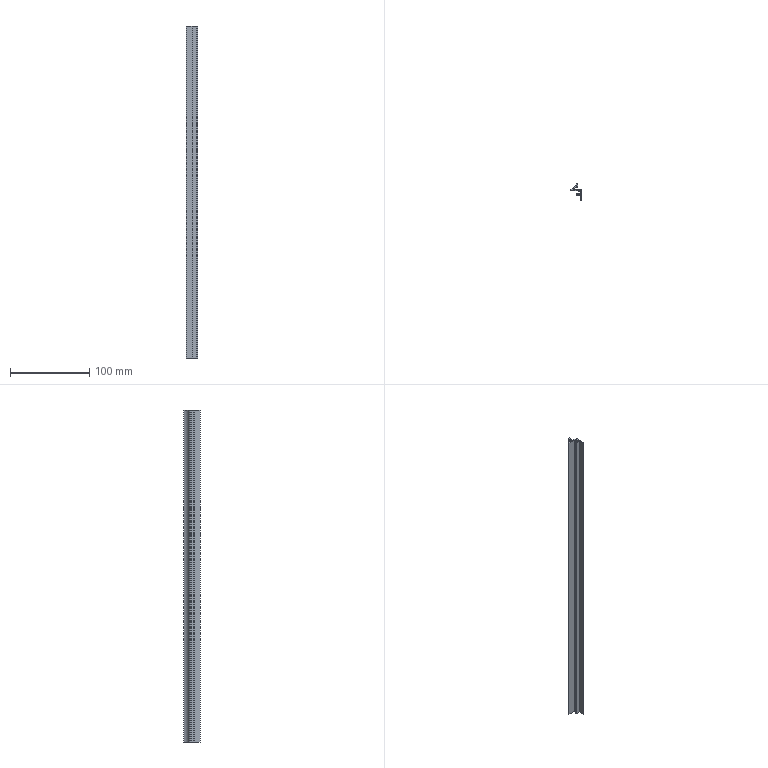Part | SolidWorks | features BaseBody 1, ICE 1, MoveFace 1 | 1 solid | 27 faces | box 14 x 20.3 x 420 mm | volume 21385 mm3 | plane 20 | cylinder 7 | commonest cylinder face diameters 0.387 x2 0.8 x2 0.4 x1 20 x1 22 x1
STEP:
#1=CARTESIAN_POINT('',(-5.304,-0.625,200.));
#2=VERTEX_POINT('',#1);
#3=CARTESIAN_POINT('',(-5.449,-0.8125,200.));
#4=VERTEX_POINT('',#3);
#5=CARTESIAN_POINT('',(-5.255,-0.8125,200.));
#6=DIRECTION('',(0.,0.,1.));
#7=DIRECTION('',(-1.,0.,0.));
#8=AXIS2_PLACEMENT_3D('',#5,#6,#7);
#9=CIRCLE('',#8,0.1937);
#10=EDGE_CURVE('',#2,#4,#9,.T.);
#11=ORIENTED_EDGE('',*,*,#10,.T.);
#12=CARTESIAN_POINT('',(-5.449,-0.8125,-220.));
#13=VERTEX_POINT('',#12);
#14=CARTESIAN_POINT('',(-5.449,-0.8125,230.));
#15=DIRECTION('',(0.,0.,-1.));
#16=VECTOR('',#15,1000.);
#17=LINE('',#14,#16);
#18=EDGE_CURVE('',#4,#13,#17,.T.);
#19=ORIENTED_EDGE('',*,*,#18,.T.);
#20=CARTESIAN_POINT('',(-5.304,-0.625,-220.));
#21=VERTEX_POINT('',#20);
#22=CARTESIAN_POINT('',(-5.255,-0.8125,-220.));
#23=DIRECTION('',(0.,0.,-1.));
#24=DIRECTION('',(1.,0.,0.));
#25=AXIS2_PLACEMENT_3D('',#22,#23,#24);
#26=CIRCLE('',#25,0.1937);
#27=EDGE_CURVE('',#13,#21,#26,.T.);
#28=ORIENTED_EDGE('',*,*,#27,.T.);
#29=CARTESIAN_POINT('',(-5.304,-0.625,230.));
#30=DIRECTION('',(0.,0.,-1.));
#31=VECTOR('',#30,1000.);
#32=LINE('',#29,#31);
#33=EDGE_CURVE('',#2,#21,#32,.T.);
#34=ORIENTED_EDGE('',*,*,#33,.F.);
#35=EDGE_LOOP('',(#11,#19,#28,#34));
#36=FACE_OUTER_BOUND('',#35,.T.);
#37=CARTESIAN_POINT('',(-5.255,-0.8125,230.));
#38=DIRECTION('',(0.,0.,-1.));
#39=DIRECTION('',(-1.,0.,0.));
#40=AXIS2_PLACEMENT_3D('',#37,#38,#39);
#41=CYLINDRICAL_SURFACE('',#40,0.1937);
#42=ADVANCED_FACE('',(#36),#41,.F.);
#43=CARTESIAN_POINT('',(5.,-1.,-220.));
#44=VERTEX_POINT('',#43);
#45=CARTESIAN_POINT('',(5.,-14.3,-220.));
#46=VERTEX_POINT('',#45);
#47=CARTESIAN_POINT('',(5.,29.623,-220.));
#48=DIRECTION('',(0.,-1.,0.));
#49=VECTOR('',#48,1000.);
#50=LINE('',#47,#49);
#51=EDGE_CURVE('',#44,#46,#50,.T.);
#52=ORIENTED_EDGE('',*,*,#51,.F.);
#53=CARTESIAN_POINT('',(5.,-1.,200.));
#54=VERTEX_POINT('',#53);
#55=CARTESIAN_POINT('',(5.,-1.,230.));
#56=DIRECTION('',(0.,0.,-1.));
#57=VECTOR('',#56,1000.);
#58=LINE('',#55,#57);
#59=EDGE_CURVE('',#54,#44,#58,.T.);
#60=ORIENTED_EDGE('',*,*,#59,.F.);
#61=CARTESIAN_POINT('',(5.,-14.3,200.));
#62=VERTEX_POINT('',#61);
#63=CARTESIAN_POINT('',(5.,-14.3,200.));
#64=DIRECTION('',(0.,1.,0.));
#65=VECTOR('',#64,1000.);
#66=LINE('',#63,#65);
#67=EDGE_CURVE('',#62,#54,#66,.T.);
#68=ORIENTED_EDGE('',*,*,#67,.F.);
#69=CARTESIAN_POINT('',(5.,-14.3,230.));
#70=DIRECTION('',(0.,0.,1.));
#71=VECTOR('',#70,1000.);
#72=LINE('',#69,#71);
#73=EDGE_CURVE('',#46,#62,#72,.T.);
#74=ORIENTED_EDGE('',*,*,#73,.F.);
#75=EDGE_LOOP('',(#52,#60,#68,#74));
#76=FACE_OUTER_BOUND('',#75,.T.);
#77=CARTESIAN_POINT('',(5.,-14.3,230.));
#78=DIRECTION('',(-1.,0.,0.));
#79=DIRECTION('',(0.,0.,1.));
#80=AXIS2_PLACEMENT_3D('',#77,#78,#79);
#81=PLANE('',#80);
#82=ADVANCED_FACE('',(#76),#81,.F.);
#83=CARTESIAN_POINT('',(-9.,-2.,-220.));
#84=VERTEX_POINT('',#83);
#85=CARTESIAN_POINT('',(-9.,-2.,200.));
#86=VERTEX_POINT('',#85);
#87=CARTESIAN_POINT('',(-9.,-2.,230.));
#88=DIRECTION('',(0.,0.,1.));
#89=VECTOR('',#88,1000.);
#90=LINE('',#87,#89);
#91=EDGE_CURVE('',#84,#86,#90,.T.);
#92=ORIENTED_EDGE('',*,*,#91,.F.);
#93=CARTESIAN_POINT('',(0.9,-2.,-220.));
#94=VERTEX_POINT('',#93);
#95=CARTESIAN_POINT('',(5.,-2.,-220.));
#96=DIRECTION('',(-1.,0.,0.));
#97=VECTOR('',#96,1000.);
#98=LINE('',#95,#97);
#99=EDGE_CURVE('',#94,#84,#98,.T.);
#100=ORIENTED_EDGE('',*,*,#99,.F.);
#101=CARTESIAN_POINT('',(0.9,-2.,200.));
#102=VERTEX_POINT('',#101);
#103=CARTESIAN_POINT('',(0.9,-2.,230.));
#104=DIRECTION('',(0.,0.,-1.));
#105=VECTOR('',#104,1000.);
#106=LINE('',#103,#105);
#107=EDGE_CURVE('',#102,#94,#106,.T.);
#108=ORIENTED_EDGE('',*,*,#107,.F.);
#109=CARTESIAN_POINT('',(5.,-2.,200.));
#110=DIRECTION('',(1.,0.,0.));
#111=VECTOR('',#110,1000.);
#112=LINE('',#109,#111);
#113=EDGE_CURVE('',#86,#102,#112,.T.);
#114=ORIENTED_EDGE('',*,*,#113,.F.);
#115=EDGE_LOOP('',(#92,#100,#108,#114));
#116=FACE_OUTER_BOUND('',#115,.T.);
#117=CARTESIAN_POINT('',(-9.,-2.,230.));
#118=DIRECTION('',(0.,1.,0.));
#119=DIRECTION('',(0.,0.,1.));
#120=AXIS2_PLACEMENT_3D('',#117,#118,#119);
#121=PLANE('',#120);
#122=ADVANCED_FACE('',(#116),#121,.F.);
#123=CARTESIAN_POINT('',(4.,-6.,200.));
#124=VERTEX_POINT('',#123);
#125=CARTESIAN_POINT('',(4.,-3.,200.));
#126=VERTEX_POINT('',#125);
#127=CARTESIAN_POINT('',(4.,29.623,200.));
#128=DIRECTION('',(0.,1.,0.));
#129=VECTOR('',#128,1000.);
#130=LINE('',#127,#129);
#131=EDGE_CURVE('',#124,#126,#130,.T.);
#132=ORIENTED_EDGE('',*,*,#131,.F.);
#133=CARTESIAN_POINT('',(1.,-6.,200.));
#134=VERTEX_POINT('',#133);
#135=CARTESIAN_POINT('',(5.,-6.,200.));
#136=DIRECTION('',(1.,0.,0.));
#137=VECTOR('',#136,1000.);
#138=LINE('',#135,#137);
#139=EDGE_CURVE('',#134,#124,#138,.T.);
#140=ORIENTED_EDGE('',*,*,#139,.F.);
#141=CARTESIAN_POINT('',(1.,-6.7,200.));
#142=VERTEX_POINT('',#141);
#143=CARTESIAN_POINT('',(1.,-6.,200.));
#144=DIRECTION('',(0.,-1.,0.));
#145=VECTOR('',#144,1000.);
#146=LINE('',#143,#145);
#147=EDGE_CURVE('',#134,#142,#146,.T.);
#148=ORIENTED_EDGE('',*,*,#147,.T.);
#149=CARTESIAN_POINT('',(-1.7,-6.7,200.));
#150=VERTEX_POINT('',#149);
#151=CARTESIAN_POINT('',(5.,-6.7,200.));
#152=DIRECTION('',(1.,0.,0.));
#153=VECTOR('',#152,1000.);
#154=LINE('',#151,#153);
#155=EDGE_CURVE('',#150,#142,#154,.T.);
#156=ORIENTED_EDGE('',*,*,#155,.F.);
#157=CARTESIAN_POINT('',(-1.7,-7.7,200.));
#158=VERTEX_POINT('',#157);
#159=CARTESIAN_POINT('',(-1.7,-6.7,200.));
#160=DIRECTION('',(0.,-1.,0.));
#161=VECTOR('',#160,1000.);
#162=LINE('',#159,#161);
#163=EDGE_CURVE('',#150,#158,#162,.T.);
#164=ORIENTED_EDGE('',*,*,#163,.T.);
#165=CARTESIAN_POINT('',(4.,-7.7,200.));
#166=VERTEX_POINT('',#165);
#167=CARTESIAN_POINT('',(5.,-7.7,200.));
#168=DIRECTION('',(-1.,0.,0.));
#169=VECTOR('',#168,1000.);
#170=LINE('',#167,#169);
#171=EDGE_CURVE('',#166,#158,#170,.T.);
#172=ORIENTED_EDGE('',*,*,#171,.F.);
#173=CARTESIAN_POINT('',(4.,-14.3,200.));
#174=VERTEX_POINT('',#173);
#175=CARTESIAN_POINT('',(4.,29.623,200.));
#176=DIRECTION('',(0.,1.,0.));
#177=VECTOR('',#176,1000.);
#178=LINE('',#175,#177);
#179=EDGE_CURVE('',#174,#166,#178,.T.);
#180=ORIENTED_EDGE('',*,*,#179,.F.);
#181=CARTESIAN_POINT('',(5.,-14.3,200.));
#182=DIRECTION('',(-1.,0.,0.));
#183=VECTOR('',#182,1000.);
#184=LINE('',#181,#183);
#185=EDGE_CURVE('',#62,#174,#184,.T.);
#186=ORIENTED_EDGE('',*,*,#185,.F.);
#187=ORIENTED_EDGE('',*,*,#67,.T.);
#188=CARTESIAN_POINT('',(-5.207,-1.,200.));
#189=VERTEX_POINT('',#188);
#190=CARTESIAN_POINT('',(5.,-1.,200.));
#191=DIRECTION('',(1.,0.,0.));
#192=VECTOR('',#191,1000.);
#193=LINE('',#190,#192);
#194=EDGE_CURVE('',#189,#54,#193,.T.);
#195=ORIENTED_EDGE('',*,*,#194,.F.);
#196=CARTESIAN_POINT('',(-5.255,-0.8125,200.));
#197=DIRECTION('',(0.,0.,1.));
#198=DIRECTION('',(-1.,0.,0.));
#199=AXIS2_PLACEMENT_3D('',#196,#197,#198);
#200=CIRCLE('',#199,0.1937);
#201=EDGE_CURVE('',#4,#189,#200,.T.);
#202=ORIENTED_EDGE('',*,*,#201,.F.);
#203=ORIENTED_EDGE('',*,*,#10,.F.);
#204=CARTESIAN_POINT('',(-1.368,3.063,200.));
#205=VERTEX_POINT('',#204);
#206=CARTESIAN_POINT('',(-10.628,9.,200.));
#207=DIRECTION('',(0.,0.,1.));
#208=DIRECTION('',(-1.,0.,0.));
#209=AXIS2_PLACEMENT_3D('',#206,#207,#208);
#210=CIRCLE('',#209,11.);
#211=EDGE_CURVE('',#2,#205,#210,.T.);
#212=ORIENTED_EDGE('',*,*,#211,.T.);
#213=CARTESIAN_POINT('',(-1.,2.955,200.));
#214=VERTEX_POINT('',#213);
#215=CARTESIAN_POINT('',(-1.2,2.955,200.));
#216=DIRECTION('',(0.,0.,1.));
#217=DIRECTION('',(-1.,0.,0.));
#218=AXIS2_PLACEMENT_3D('',#215,#216,#217);
#219=CIRCLE('',#218,0.2);
#220=EDGE_CURVE('',#214,#205,#219,.T.);
#221=ORIENTED_EDGE('',*,*,#220,.F.);
#222=CARTESIAN_POINT('',(-1.,1.5,200.));
#223=VERTEX_POINT('',#222);
#224=CARTESIAN_POINT('',(-1.,2.955,200.));
#225=DIRECTION('',(0.,1.,0.));
#226=VECTOR('',#225,1000.);
#227=LINE('',#224,#226);
#228=EDGE_CURVE('',#223,#214,#227,.T.);
#229=ORIENTED_EDGE('',*,*,#228,.F.);
#230=CARTESIAN_POINT('',(0.,1.5,200.));
#231=VERTEX_POINT('',#230);
#232=CARTESIAN_POINT('',(-1.,1.5,200.));
#233=DIRECTION('',(-1.,0.,0.));
#234=VECTOR('',#233,1000.);
#235=LINE('',#232,#234);
#236=EDGE_CURVE('',#231,#223,#235,.T.);
#237=ORIENTED_EDGE('',*,*,#236,.F.);
#238=CARTESIAN_POINT('',(0.,6.,200.));
#239=VERTEX_POINT('',#238);
#240=CARTESIAN_POINT('',(0.,1.5,200.));
#241=DIRECTION('',(0.,-1.,0.));
#242=VECTOR('',#241,1000.);
#243=LINE('',#240,#242);
#244=EDGE_CURVE('',#239,#231,#243,.T.);
#245=ORIENTED_EDGE('',*,*,#244,.F.);
#246=CARTESIAN_POINT('',(-0.8,6.,200.));
#247=VERTEX_POINT('',#246);
#248=CARTESIAN_POINT('',(0.,6.,200.));
#249=DIRECTION('',(1.,0.,0.));
#250=VECTOR('',#249,1000.);
#251=LINE('',#248,#250);
#252=EDGE_CURVE('',#247,#239,#251,.T.);
#253=ORIENTED_EDGE('',*,*,#252,.F.);
#254=CARTESIAN_POINT('',(-1.178,5.731,200.));
#255=VERTEX_POINT('',#254);
#256=CARTESIAN_POINT('',(-0.8,5.6,200.));
#257=DIRECTION('',(0.,0.,1.));
#258=DIRECTION('',(-1.,0.,0.));
#259=AXIS2_PLACEMENT_3D('',#256,#257,#258);
#260=CIRCLE('',#259,0.4);
#261=EDGE_CURVE('',#247,#255,#260,.T.);
#262=ORIENTED_EDGE('',*,*,#261,.T.);
#263=CARTESIAN_POINT('',(-8.678,-0.8077,200.));
#264=VERTEX_POINT('',#263);
#265=CARTESIAN_POINT('',(-10.628,9.,200.));
#266=DIRECTION('',(0.,0.,1.));
#267=DIRECTION('',(-1.,0.,0.));
#268=AXIS2_PLACEMENT_3D('',#265,#266,#267);
#269=CIRCLE('',#268,10.);
#270=EDGE_CURVE('',#264,#255,#269,.T.);
#271=ORIENTED_EDGE('',*,*,#270,.F.);
#272=CARTESIAN_POINT('',(-9.,-1.2,200.));
#273=VERTEX_POINT('',#272);
#274=CARTESIAN_POINT('',(-8.6,-1.2,200.));
#275=DIRECTION('',(0.,0.,1.));
#276=DIRECTION('',(-1.,0.,0.));
#277=AXIS2_PLACEMENT_3D('',#274,#275,#276);
#278=CIRCLE('',#277,0.4);
#279=EDGE_CURVE('',#264,#273,#278,.T.);
#280=ORIENTED_EDGE('',*,*,#279,.T.);
#281=CARTESIAN_POINT('',(-9.,8.,200.));
#282=DIRECTION('',(0.,-1.,0.));
#283=VECTOR('',#282,1000.);
#284=LINE('',#281,#283);
#285=EDGE_CURVE('',#273,#86,#284,.T.);
#286=ORIENTED_EDGE('',*,*,#285,.T.);
#287=ORIENTED_EDGE('',*,*,#113,.T.);
#288=CARTESIAN_POINT('',(0.9,-3.,200.));
#289=VERTEX_POINT('',#288);
#290=CARTESIAN_POINT('',(0.9,29.623,200.));
#291=DIRECTION('',(0.,1.,0.));
#292=VECTOR('',#291,1000.);
#293=LINE('',#290,#292);
#294=EDGE_CURVE('',#289,#102,#293,.T.);
#295=ORIENTED_EDGE('',*,*,#294,.F.);
#296=CARTESIAN_POINT('',(5.,-3.,200.));
#297=DIRECTION('',(-1.,0.,0.));
#298=VECTOR('',#297,1000.);
#299=LINE('',#296,#298);
#300=EDGE_CURVE('',#126,#289,#299,.T.);
#301=ORIENTED_EDGE('',*,*,#300,.F.);
#302=EDGE_LOOP('',(#132,#140,#148,#156,#164,#172,#180,#186,#187,#195,#202,#203,#212,#221,#229,#237,#245,#253,#262,#271,#280,#286,#287,#295,#301));
#303=FACE_OUTER_BOUND('',#302,.T.);
#304=CARTESIAN_POINT('',(5.,29.623,200.));
#305=DIRECTION('',(0.,0.,-1.));
#306=DIRECTION('',(-1.,0.,0.));
#307=AXIS2_PLACEMENT_3D('',#304,#305,#306);
#308=PLANE('',#307);
#309=ADVANCED_FACE('',(#303),#308,.F.);
#310=ORIENTED_EDGE('',*,*,#185,.T.);
#311=CARTESIAN_POINT('',(4.,-14.3,-220.));
#312=VERTEX_POINT('',#311);
#313=CARTESIAN_POINT('',(4.,-14.3,230.));
#314=DIRECTION('',(0.,0.,1.));
#315=VECTOR('',#314,1000.);
#316=LINE('',#313,#315);
#317=EDGE_CURVE('',#312,#174,#316,.T.);
#318=ORIENTED_EDGE('',*,*,#317,.F.);
#319=CARTESIAN_POINT('',(5.,-14.3,-220.));
#320=DIRECTION('',(-1.,0.,0.));
#321=VECTOR('',#320,1000.);
#322=LINE('',#319,#321);
#323=EDGE_CURVE('',#46,#312,#322,.T.);
#324=ORIENTED_EDGE('',*,*,#323,.F.);
#325=ORIENTED_EDGE('',*,*,#73,.T.);
#326=EDGE_LOOP('',(#310,#318,#324,#325));
#327=FACE_OUTER_BOUND('',#326,.T.);
#328=CARTESIAN_POINT('',(4.,-14.3,230.));
#329=DIRECTION('',(0.,1.,0.));
#330=DIRECTION('',(0.,0.,1.));
#331=AXIS2_PLACEMENT_3D('',#328,#329,#330);
#332=PLANE('',#331);
#333=ADVANCED_FACE('',(#327),#332,.F.);
#334=ORIENTED_EDGE('',*,*,#51,.T.);
#335=ORIENTED_EDGE('',*,*,#323,.T.);
#336=CARTESIAN_POINT('',(4.,-7.7,-220.));
#337=VERTEX_POINT('',#336);
#338=CARTESIAN_POINT('',(4.,-7.7,-220.));
#339=DIRECTION('',(0.,-1.,0.));
#340=VECTOR('',#339,1000.);
#341=LINE('',#338,#340);
#342=EDGE_CURVE('',#337,#312,#341,.T.);
#343=ORIENTED_EDGE('',*,*,#342,.F.);
#344=CARTESIAN_POINT('',(-1.7,-7.7,-220.));
#345=VERTEX_POINT('',#344);
#346=CARTESIAN_POINT('',(-1.7,-7.7,-220.));
#347=DIRECTION('',(1.,0.,0.));
#348=VECTOR('',#347,1000.);
#349=LINE('',#346,#348);
#350=EDGE_CURVE('',#345,#337,#349,.T.);
#351=ORIENTED_EDGE('',*,*,#350,.F.);
#352=CARTESIAN_POINT('',(-1.7,-6.7,-220.));
#353=VERTEX_POINT('',#352);
#354=CARTESIAN_POINT('',(-1.7,29.623,-220.));
#355=DIRECTION('',(0.,1.,0.));
#356=VECTOR('',#355,1000.);
#357=LINE('',#354,#356);
#358=EDGE_CURVE('',#345,#353,#357,.T.);
#359=ORIENTED_EDGE('',*,*,#358,.T.);
#360=CARTESIAN_POINT('',(1.,-6.7,-220.));
#361=VERTEX_POINT('',#360);
#362=CARTESIAN_POINT('',(1.,-6.7,-220.));
#363=DIRECTION('',(-1.,0.,0.));
#364=VECTOR('',#363,1000.);
#365=LINE('',#362,#364);
#366=EDGE_CURVE('',#361,#353,#365,.T.);
#367=ORIENTED_EDGE('',*,*,#366,.F.);
#368=CARTESIAN_POINT('',(1.,-6.,-220.));
#369=VERTEX_POINT('',#368);
#370=CARTESIAN_POINT('',(1.,29.623,-220.));
#371=DIRECTION('',(0.,1.,0.));
#372=VECTOR('',#371,1000.);
#373=LINE('',#370,#372);
#374=EDGE_CURVE('',#361,#369,#373,.T.);
#375=ORIENTED_EDGE('',*,*,#374,.T.);
#376=CARTESIAN_POINT('',(4.,-6.,-220.));
#377=VERTEX_POINT('',#376);
#378=CARTESIAN_POINT('',(4.,-6.,-220.));
#379=DIRECTION('',(-1.,0.,0.));
#380=VECTOR('',#379,1000.);
#381=LINE('',#378,#380);
#382=EDGE_CURVE('',#377,#369,#381,.T.);
#383=ORIENTED_EDGE('',*,*,#382,.F.);
#384=CARTESIAN_POINT('',(4.,-3.,-220.));
#385=VERTEX_POINT('',#384);
#386=CARTESIAN_POINT('',(4.,-3.,-220.));
#387=DIRECTION('',(0.,-1.,0.));
#388=VECTOR('',#387,1000.);
#389=LINE('',#386,#388);
#390=EDGE_CURVE('',#385,#377,#389,.T.);
#391=ORIENTED_EDGE('',*,*,#390,.F.);
#392=CARTESIAN_POINT('',(0.9,-3.,-220.));
#393=VERTEX_POINT('',#392);
#394=CARTESIAN_POINT('',(0.9,-3.,-220.));
#395=DIRECTION('',(1.,0.,0.));
#396=VECTOR('',#395,1000.);
#397=LINE('',#394,#396);
#398=EDGE_CURVE('',#393,#385,#397,.T.);
#399=ORIENTED_EDGE('',*,*,#398,.F.);
#400=CARTESIAN_POINT('',(0.9,-2.,-220.));
#401=DIRECTION('',(0.,-1.,0.));
#402=VECTOR('',#401,1000.);
#403=LINE('',#400,#402);
#404=EDGE_CURVE('',#94,#393,#403,.T.);
#405=ORIENTED_EDGE('',*,*,#404,.F.);
#406=ORIENTED_EDGE('',*,*,#99,.T.);
#407=CARTESIAN_POINT('',(-9.,-1.2,-220.));
#408=VERTEX_POINT('',#407);
#409=CARTESIAN_POINT('',(-9.,-1.2,-220.));
#410=DIRECTION('',(0.,-1.,0.));
#411=VECTOR('',#410,1000.);
#412=LINE('',#409,#411);
#413=EDGE_CURVE('',#408,#84,#412,.T.);
#414=ORIENTED_EDGE('',*,*,#413,.F.);
#415=CARTESIAN_POINT('',(-8.678,-0.8077,-220.));
#416=VERTEX_POINT('',#415);
#417=CARTESIAN_POINT('',(-8.6,-1.2,-220.));
#418=DIRECTION('',(0.,0.,-1.));
#419=DIRECTION('',(1.,0.,0.));
#420=AXIS2_PLACEMENT_3D('',#417,#418,#419);
#421=CIRCLE('',#420,0.4);
#422=EDGE_CURVE('',#408,#416,#421,.T.);
#423=ORIENTED_EDGE('',*,*,#422,.T.);
#424=CARTESIAN_POINT('',(-1.178,5.731,-220.));
#425=VERTEX_POINT('',#424);
#426=CARTESIAN_POINT('',(-10.628,9.,-220.));
#427=DIRECTION('',(0.,0.,-1.));
#428=DIRECTION('',(1.,0.,0.));
#429=AXIS2_PLACEMENT_3D('',#426,#427,#428);
#430=CIRCLE('',#429,10.);
#431=EDGE_CURVE('',#425,#416,#430,.T.);
#432=ORIENTED_EDGE('',*,*,#431,.F.);
#433=CARTESIAN_POINT('',(-0.8,6.,-220.));
#434=VERTEX_POINT('',#433);
#435=CARTESIAN_POINT('',(-0.8,5.6,-220.));
#436=DIRECTION('',(0.,0.,-1.));
#437=DIRECTION('',(1.,0.,0.));
#438=AXIS2_PLACEMENT_3D('',#435,#436,#437);
#439=CIRCLE('',#438,0.4);
#440=EDGE_CURVE('',#425,#434,#439,.T.);
#441=ORIENTED_EDGE('',*,*,#440,.T.);
#442=CARTESIAN_POINT('',(0.,6.,-220.));
#443=VERTEX_POINT('',#442);
#444=CARTESIAN_POINT('',(0.,6.,-220.));
#445=DIRECTION('',(-1.,0.,0.));
#446=VECTOR('',#445,1000.);
#447=LINE('',#444,#446);
#448=EDGE_CURVE('',#443,#434,#447,.T.);
#449=ORIENTED_EDGE('',*,*,#448,.F.);
#450=CARTESIAN_POINT('',(0.,1.5,-220.));
#451=VERTEX_POINT('',#450);
#452=CARTESIAN_POINT('',(0.,1.5,-220.));
#453=DIRECTION('',(0.,1.,0.));
#454=VECTOR('',#453,1000.);
#455=LINE('',#452,#454);
#456=EDGE_CURVE('',#451,#443,#455,.T.);
#457=ORIENTED_EDGE('',*,*,#456,.F.);
#458=CARTESIAN_POINT('',(-1.,1.5,-220.));
#459=VERTEX_POINT('',#458);
#460=CARTESIAN_POINT('',(-1.,1.5,-220.));
#461=DIRECTION('',(1.,0.,0.));
#462=VECTOR('',#461,1000.);
#463=LINE('',#460,#462);
#464=EDGE_CURVE('',#459,#451,#463,.T.);
#465=ORIENTED_EDGE('',*,*,#464,.F.);
#466=CARTESIAN_POINT('',(-1.,2.955,-220.));
#467=VERTEX_POINT('',#466);
#468=CARTESIAN_POINT('',(-1.,2.955,-220.));
#469=DIRECTION('',(0.,-1.,0.));
#470=VECTOR('',#469,1000.);
#471=LINE('',#468,#470);
#472=EDGE_CURVE('',#467,#459,#471,.T.);
#473=ORIENTED_EDGE('',*,*,#472,.F.);
#474=CARTESIAN_POINT('',(-1.368,3.063,-220.));
#475=VERTEX_POINT('',#474);
#476=CARTESIAN_POINT('',(-1.2,2.955,-220.));
#477=DIRECTION('',(0.,0.,-1.));
#478=DIRECTION('',(1.,0.,0.));
#479=AXIS2_PLACEMENT_3D('',#476,#477,#478);
#480=CIRCLE('',#479,0.2);
#481=EDGE_CURVE('',#475,#467,#480,.T.);
#482=ORIENTED_EDGE('',*,*,#481,.F.);
#483=CARTESIAN_POINT('',(-10.628,9.,-220.));
#484=DIRECTION('',(0.,0.,-1.));
#485=DIRECTION('',(1.,0.,0.));
#486=AXIS2_PLACEMENT_3D('',#483,#484,#485);
#487=CIRCLE('',#486,11.);
#488=EDGE_CURVE('',#475,#21,#487,.T.);
#489=ORIENTED_EDGE('',*,*,#488,.T.);
#490=ORIENTED_EDGE('',*,*,#27,.F.);
#491=CARTESIAN_POINT('',(-5.207,-1.,-220.));
#492=VERTEX_POINT('',#491);
#493=CARTESIAN_POINT('',(-5.255,-0.8125,-220.));
#494=DIRECTION('',(0.,0.,-1.));
#495=DIRECTION('',(1.,0.,0.));
#496=AXIS2_PLACEMENT_3D('',#493,#494,#495);
#497=CIRCLE('',#496,0.1937);
#498=EDGE_CURVE('',#492,#13,#497,.T.);
#499=ORIENTED_EDGE('',*,*,#498,.F.);
#500=CARTESIAN_POINT('',(5.,-1.,-220.));
#501=DIRECTION('',(-1.,0.,0.));
#502=VECTOR('',#501,1000.);
#503=LINE('',#500,#502);
#504=EDGE_CURVE('',#44,#492,#503,.T.);
#505=ORIENTED_EDGE('',*,*,#504,.F.);
#506=EDGE_LOOP('',(#334,#335,#343,#351,#359,#367,#375,#383,#391,#399,#405,#406,#414,#423,#432,#441,#449,#457,#465,#473,#482,#489,#490,#499,#505));
#507=FACE_OUTER_BOUND('',#506,.T.);
#508=CARTESIAN_POINT('',(5.,29.623,-220.));
#509=DIRECTION('',(0.,0.,1.));
#510=DIRECTION('',(1.,0.,0.));
#511=AXIS2_PLACEMENT_3D('',#508,#509,#510);
#512=PLANE('',#511);
#513=ADVANCED_FACE('',(#507),#512,.F.);
#514=ORIENTED_EDGE('',*,*,#59,.T.);
#515=ORIENTED_EDGE('',*,*,#504,.T.);
#516=CARTESIAN_POINT('',(-5.207,-1.,230.));
#517=DIRECTION('',(0.,0.,-1.));
#518=VECTOR('',#517,1000.);
#519=LINE('',#516,#518);
#520=EDGE_CURVE('',#189,#492,#519,.T.);
#521=ORIENTED_EDGE('',*,*,#520,.F.);
#522=ORIENTED_EDGE('',*,*,#194,.T.);
#523=EDGE_LOOP('',(#514,#515,#521,#522));
#524=FACE_OUTER_BOUND('',#523,.T.);
#525=CARTESIAN_POINT('',(5.,-1.,230.));
#526=DIRECTION('',(0.,-1.,0.));
#527=DIRECTION('',(0.,0.,-1.));
#528=AXIS2_PLACEMENT_3D('',#525,#526,#527);
#529=PLANE('',#528);
#530=ADVANCED_FACE('',(#524),#529,.F.);
#531=CARTESIAN_POINT('',(-9.,-1.2,230.));
#532=DIRECTION('',(0.,0.,1.));
#533=VECTOR('',#532,1000.);
#534=LINE('',#531,#533);
#535=EDGE_CURVE('',#408,#273,#534,.T.);
#536=ORIENTED_EDGE('',*,*,#535,.F.);
#537=ORIENTED_EDGE('',*,*,#413,.T.);
#538=ORIENTED_EDGE('',*,*,#91,.T.);
#539=ORIENTED_EDGE('',*,*,#285,.F.);
#540=EDGE_LOOP('',(#536,#537,#538,#539));
#541=FACE_OUTER_BOUND('',#540,.T.);
#542=CARTESIAN_POINT('',(-9.,-1.2,230.));
#543=DIRECTION('',(1.,0.,0.));
#544=DIRECTION('',(0.,0.,-1.));
#545=AXIS2_PLACEMENT_3D('',#542,#543,#544);
#546=PLANE('',#545);
#547=ADVANCED_FACE('',(#541),#546,.F.);
#548=ORIENTED_EDGE('',*,*,#294,.T.);
#549=ORIENTED_EDGE('',*,*,#107,.T.);
#550=ORIENTED_EDGE('',*,*,#404,.T.);
#551=CARTESIAN_POINT('',(0.9,-3.,230.));
#552=DIRECTION('',(0.,0.,-1.));
#553=VECTOR('',#552,1000.);
#554=LINE('',#551,#553);
#555=EDGE_CURVE('',#289,#393,#554,.T.);
#556=ORIENTED_EDGE('',*,*,#555,.F.);
#557=EDGE_LOOP('',(#548,#549,#550,#556));
#558=FACE_OUTER_BOUND('',#557,.T.);
#559=CARTESIAN_POINT('',(0.9,-2.,230.));
#560=DIRECTION('',(1.,0.,0.));
#561=DIRECTION('',(0.,0.,-1.));
#562=AXIS2_PLACEMENT_3D('',#559,#560,#561);
#563=PLANE('',#562);
#564=ADVANCED_FACE('',(#558),#563,.F.);
#565=ORIENTED_EDGE('',*,*,#300,.T.);
#566=ORIENTED_EDGE('',*,*,#555,.T.);
#567=ORIENTED_EDGE('',*,*,#398,.T.);
#568=CARTESIAN_POINT('',(4.,-3.,230.));
#569=DIRECTION('',(0.,0.,-1.));
#570=VECTOR('',#569,1000.);
#571=LINE('',#568,#570);
#572=EDGE_CURVE('',#126,#385,#571,.T.);
#573=ORIENTED_EDGE('',*,*,#572,.F.);
#574=EDGE_LOOP('',(#565,#566,#567,#573));
#575=FACE_OUTER_BOUND('',#574,.T.);
#576=CARTESIAN_POINT('',(0.9,-3.,230.));
#577=DIRECTION('',(0.,1.,0.));
#578=DIRECTION('',(0.,0.,1.));
#579=AXIS2_PLACEMENT_3D('',#576,#577,#578);
#580=PLANE('',#579);
#581=ADVANCED_FACE('',(#575),#580,.F.);
#582=ORIENTED_EDGE('',*,*,#131,.T.);
#583=ORIENTED_EDGE('',*,*,#572,.T.);
#584=ORIENTED_EDGE('',*,*,#390,.T.);
#585=CARTESIAN_POINT('',(4.,-6.,230.));
#586=DIRECTION('',(0.,0.,-1.));
#587=VECTOR('',#586,1000.);
#588=LINE('',#585,#587);
#589=EDGE_CURVE('',#124,#377,#588,.T.);
#590=ORIENTED_EDGE('',*,*,#589,.F.);
#591=EDGE_LOOP('',(#582,#583,#584,#590));
#592=FACE_OUTER_BOUND('',#591,.T.);
#593=CARTESIAN_POINT('',(4.,-3.,230.));
#594=DIRECTION('',(1.,0.,0.));
#595=DIRECTION('',(0.,0.,-1.));
#596=AXIS2_PLACEMENT_3D('',#593,#594,#595);
#597=PLANE('',#596);
#598=ADVANCED_FACE('',(#592),#597,.F.);
#599=ORIENTED_EDGE('',*,*,#139,.T.);
#600=ORIENTED_EDGE('',*,*,#589,.T.);
#601=ORIENTED_EDGE('',*,*,#382,.T.);
#602=CARTESIAN_POINT('',(1.,-6.,230.));
#603=DIRECTION('',(0.,0.,-1.));
#604=VECTOR('',#603,1000.);
#605=LINE('',#602,#604);
#606=EDGE_CURVE('',#134,#369,#605,.T.);
#607=ORIENTED_EDGE('',*,*,#606,.F.);
#608=EDGE_LOOP('',(#599,#600,#601,#607));
#609=FACE_OUTER_BOUND('',#608,.T.);
#610=CARTESIAN_POINT('',(4.,-6.,230.));
#611=DIRECTION('',(0.,-1.,0.));
#612=DIRECTION('',(0.,0.,-1.));
#613=AXIS2_PLACEMENT_3D('',#610,#611,#612);
#614=PLANE('',#613);
#615=ADVANCED_FACE('',(#609),#614,.F.);
#616=ORIENTED_EDGE('',*,*,#155,.T.);
#617=CARTESIAN_POINT('',(1.,-6.7,230.));
#618=DIRECTION('',(0.,0.,1.));
#619=VECTOR('',#618,1000.);
#620=LINE('',#617,#619);
#621=EDGE_CURVE('',#361,#142,#620,.T.);
#622=ORIENTED_EDGE('',*,*,#621,.F.);
#623=ORIENTED_EDGE('',*,*,#366,.T.);
#624=CARTESIAN_POINT('',(-1.7,-6.7,230.));
#625=DIRECTION('',(0.,0.,-1.));
#626=VECTOR('',#625,1000.);
#627=LINE('',#624,#626);
#628=EDGE_CURVE('',#150,#353,#627,.T.);
#629=ORIENTED_EDGE('',*,*,#628,.F.);
#630=EDGE_LOOP('',(#616,#622,#623,#629));
#631=FACE_OUTER_BOUND('',#630,.T.);
#632=CARTESIAN_POINT('',(1.,-6.7,230.));
#633=DIRECTION('',(0.,-1.,0.));
#634=DIRECTION('',(0.,0.,-1.));
#635=AXIS2_PLACEMENT_3D('',#632,#633,#634);
#636=PLANE('',#635);
#637=ADVANCED_FACE('',(#631),#636,.F.);
#638=ORIENTED_EDGE('',*,*,#171,.T.);
#639=CARTESIAN_POINT('',(-1.7,-7.7,230.));
#640=DIRECTION('',(0.,0.,1.));
#641=VECTOR('',#640,1000.);
#642=LINE('',#639,#641);
#643=EDGE_CURVE('',#345,#158,#642,.T.);
#644=ORIENTED_EDGE('',*,*,#643,.F.);
#645=ORIENTED_EDGE('',*,*,#350,.T.);
#646=CARTESIAN_POINT('',(4.,-7.7,230.));
#647=DIRECTION('',(0.,0.,-1.));
#648=VECTOR('',#647,1000.);
#649=LINE('',#646,#648);
#650=EDGE_CURVE('',#166,#337,#649,.T.);
#651=ORIENTED_EDGE('',*,*,#650,.F.);
#652=EDGE_LOOP('',(#638,#644,#645,#651));
#653=FACE_OUTER_BOUND('',#652,.T.);
#654=CARTESIAN_POINT('',(-1.7,-7.7,230.));
#655=DIRECTION('',(0.,1.,0.));
#656=DIRECTION('',(0.,0.,1.));
#657=AXIS2_PLACEMENT_3D('',#654,#655,#656);
#658=PLANE('',#657);
#659=ADVANCED_FACE('',(#653),#658,.F.);
#660=ORIENTED_EDGE('',*,*,#179,.T.);
#661=ORIENTED_EDGE('',*,*,#650,.T.);
#662=ORIENTED_EDGE('',*,*,#342,.T.);
#663=ORIENTED_EDGE('',*,*,#317,.T.);
#664=EDGE_LOOP('',(#660,#661,#662,#663));
#665=FACE_OUTER_BOUND('',#664,.T.);
#666=CARTESIAN_POINT('',(4.,-7.7,230.));
#667=DIRECTION('',(1.,0.,0.));
#668=DIRECTION('',(0.,0.,-1.));
#669=AXIS2_PLACEMENT_3D('',#666,#667,#668);
#670=PLANE('',#669);
#671=ADVANCED_FACE('',(#665),#670,.F.);
#672=ORIENTED_EDGE('',*,*,#18,.F.);
#673=ORIENTED_EDGE('',*,*,#201,.T.);
#674=ORIENTED_EDGE('',*,*,#520,.T.);
#675=ORIENTED_EDGE('',*,*,#498,.T.);
#676=EDGE_LOOP('',(#672,#673,#674,#675));
#677=FACE_OUTER_BOUND('',#676,.T.);
#678=CARTESIAN_POINT('',(-5.255,-0.8125,230.));
#679=DIRECTION('',(0.,0.,-1.));
#680=DIRECTION('',(-1.,0.,0.));
#681=AXIS2_PLACEMENT_3D('',#678,#679,#680);
#682=CYLINDRICAL_SURFACE('',#681,0.1937);
#683=ADVANCED_FACE('',(#677),#682,.F.);
#684=CARTESIAN_POINT('',(-1.,2.955,230.));
#685=DIRECTION('',(0.,0.,1.));
#686=VECTOR('',#685,1000.);
#687=LINE('',#684,#686);
#688=EDGE_CURVE('',#467,#214,#687,.T.);
#689=ORIENTED_EDGE('',*,*,#688,.F.);
#690=ORIENTED_EDGE('',*,*,#472,.T.);
#691=CARTESIAN_POINT('',(-1.,1.5,230.));
#692=DIRECTION('',(0.,0.,-1.));
#693=VECTOR('',#692,1000.);
#694=LINE('',#691,#693);
#695=EDGE_CURVE('',#223,#459,#694,.T.);
#696=ORIENTED_EDGE('',*,*,#695,.F.);
#697=ORIENTED_EDGE('',*,*,#228,.T.);
#698=EDGE_LOOP('',(#689,#690,#696,#697));
#699=FACE_OUTER_BOUND('',#698,.T.);
#700=CARTESIAN_POINT('',(-1.,2.955,230.));
#701=DIRECTION('',(1.,0.,0.));
#702=DIRECTION('',(0.,0.,-1.));
#703=AXIS2_PLACEMENT_3D('',#700,#701,#702);
#704=PLANE('',#703);
#705=ADVANCED_FACE('',(#699),#704,.F.);
#706=ORIENTED_EDGE('',*,*,#488,.F.);
#707=CARTESIAN_POINT('',(-1.368,3.063,230.));
#708=DIRECTION('',(0.,0.,1.));
#709=VECTOR('',#708,1000.);
#710=LINE('',#707,#709);
#711=EDGE_CURVE('',#475,#205,#710,.T.);
#712=ORIENTED_EDGE('',*,*,#711,.T.);
#713=ORIENTED_EDGE('',*,*,#211,.F.);
#714=ORIENTED_EDGE('',*,*,#33,.T.);
#715=EDGE_LOOP('',(#706,#712,#713,#714));
#716=FACE_OUTER_BOUND('',#715,.T.);
#717=CARTESIAN_POINT('',(-10.628,9.,230.));
#718=DIRECTION('',(0.,0.,-1.));
#719=DIRECTION('',(-1.,0.,0.));
#720=AXIS2_PLACEMENT_3D('',#717,#718,#719);
#721=CYLINDRICAL_SURFACE('',#720,11.);
#722=ADVANCED_FACE('',(#716),#721,.T.);
#723=CARTESIAN_POINT('',(-1.178,5.731,230.));
#724=DIRECTION('',(0.,0.,1.));
#725=VECTOR('',#724,1000.);
#726=LINE('',#723,#725);
#727=EDGE_CURVE('',#425,#255,#726,.T.);
#728=ORIENTED_EDGE('',*,*,#727,.F.);
#729=ORIENTED_EDGE('',*,*,#431,.T.);
#730=CARTESIAN_POINT('',(-8.678,-0.8077,230.));
#731=DIRECTION('',(0.,0.,-1.));
#732=VECTOR('',#731,1000.);
#733=LINE('',#730,#732);
#734=EDGE_CURVE('',#264,#416,#733,.T.);
#735=ORIENTED_EDGE('',*,*,#734,.F.);
#736=ORIENTED_EDGE('',*,*,#270,.T.);
#737=EDGE_LOOP('',(#728,#729,#735,#736));
#738=FACE_OUTER_BOUND('',#737,.T.);
#739=CARTESIAN_POINT('',(-10.628,9.,230.));
#740=DIRECTION('',(0.,0.,-1.));
#741=DIRECTION('',(-1.,0.,0.));
#742=AXIS2_PLACEMENT_3D('',#739,#740,#741);
#743=CYLINDRICAL_SURFACE('',#742,10.);
#744=ADVANCED_FACE('',(#738),#743,.F.);
#745=CARTESIAN_POINT('',(0.,1.5,230.));
#746=DIRECTION('',(0.,0.,1.));
#747=VECTOR('',#746,1000.);
#748=LINE('',#745,#747);
#749=EDGE_CURVE('',#451,#231,#748,.T.);
#750=ORIENTED_EDGE('',*,*,#749,.F.);
#751=ORIENTED_EDGE('',*,*,#456,.T.);
#752=CARTESIAN_POINT('',(0.,6.,230.));
#753=DIRECTION('',(0.,0.,-1.));
#754=VECTOR('',#753,1000.);
#755=LINE('',#752,#754);
#756=EDGE_CURVE('',#239,#443,#755,.T.);
#757=ORIENTED_EDGE('',*,*,#756,.F.);
#758=ORIENTED_EDGE('',*,*,#244,.T.);
#759=EDGE_LOOP('',(#750,#751,#757,#758));
#760=FACE_OUTER_BOUND('',#759,.T.);
#761=CARTESIAN_POINT('',(0.,1.5,230.));
#762=DIRECTION('',(-1.,0.,0.));
#763=DIRECTION('',(0.,0.,1.));
#764=AXIS2_PLACEMENT_3D('',#761,#762,#763);
#765=PLANE('',#764);
#766=ADVANCED_FACE('',(#760),#765,.F.);
#767=ORIENTED_EDGE('',*,*,#422,.F.);
#768=ORIENTED_EDGE('',*,*,#535,.T.);
#769=ORIENTED_EDGE('',*,*,#279,.F.);
#770=ORIENTED_EDGE('',*,*,#734,.T.);
#771=EDGE_LOOP('',(#767,#768,#769,#770));
#772=FACE_OUTER_BOUND('',#771,.T.);
#773=CARTESIAN_POINT('',(-8.6,-1.2,230.));
#774=DIRECTION('',(0.,0.,-1.));
#775=DIRECTION('',(-1.,0.,0.));
#776=AXIS2_PLACEMENT_3D('',#773,#774,#775);
#777=CYLINDRICAL_SURFACE('',#776,0.4);
#778=ADVANCED_FACE('',(#772),#777,.T.);
#779=ORIENTED_EDGE('',*,*,#147,.F.);
#780=ORIENTED_EDGE('',*,*,#606,.T.);
#781=ORIENTED_EDGE('',*,*,#374,.F.);
#782=ORIENTED_EDGE('',*,*,#621,.T.);
#783=EDGE_LOOP('',(#779,#780,#781,#782));
#784=FACE_OUTER_BOUND('',#783,.T.);
#785=CARTESIAN_POINT('',(1.,-6.,230.));
#786=DIRECTION('',(1.,0.,0.));
#787=DIRECTION('',(0.,0.,-1.));
#788=AXIS2_PLACEMENT_3D('',#785,#786,#787);
#789=PLANE('',#788);
#790=ADVANCED_FACE('',(#784),#789,.F.);
#791=ORIENTED_EDGE('',*,*,#163,.F.);
#792=ORIENTED_EDGE('',*,*,#628,.T.);
#793=ORIENTED_EDGE('',*,*,#358,.F.);
#794=ORIENTED_EDGE('',*,*,#643,.T.);
#795=EDGE_LOOP('',(#791,#792,#793,#794));
#796=FACE_OUTER_BOUND('',#795,.T.);
#797=CARTESIAN_POINT('',(-1.7,-6.7,230.));
#798=DIRECTION('',(1.,0.,0.));
#799=DIRECTION('',(0.,0.,-1.));
#800=AXIS2_PLACEMENT_3D('',#797,#798,#799);
#801=PLANE('',#800);
#802=ADVANCED_FACE('',(#796),#801,.F.);
#803=ORIENTED_EDGE('',*,*,#711,.F.);
#804=ORIENTED_EDGE('',*,*,#481,.T.);
#805=ORIENTED_EDGE('',*,*,#688,.T.);
#806=ORIENTED_EDGE('',*,*,#220,.T.);
#807=EDGE_LOOP('',(#803,#804,#805,#806));
#808=FACE_OUTER_BOUND('',#807,.T.);
#809=CARTESIAN_POINT('',(-1.2,2.955,230.));
#810=DIRECTION('',(0.,0.,-1.));
#811=DIRECTION('',(-1.,0.,0.));
#812=AXIS2_PLACEMENT_3D('',#809,#810,#811);
#813=CYLINDRICAL_SURFACE('',#812,0.2);
#814=ADVANCED_FACE('',(#808),#813,.F.);
#815=ORIENTED_EDGE('',*,*,#695,.T.);
#816=ORIENTED_EDGE('',*,*,#464,.T.);
#817=ORIENTED_EDGE('',*,*,#749,.T.);
#818=ORIENTED_EDGE('',*,*,#236,.T.);
#819=EDGE_LOOP('',(#815,#816,#817,#818));
#820=FACE_OUTER_BOUND('',#819,.T.);
#821=CARTESIAN_POINT('',(-1.,1.5,230.));
#822=DIRECTION('',(0.,1.,0.));
#823=DIRECTION('',(0.,0.,1.));
#824=AXIS2_PLACEMENT_3D('',#821,#822,#823);
#825=PLANE('',#824);
#826=ADVANCED_FACE('',(#820),#825,.F.);
#827=ORIENTED_EDGE('',*,*,#440,.F.);
#828=ORIENTED_EDGE('',*,*,#727,.T.);
#829=ORIENTED_EDGE('',*,*,#261,.F.);
#830=CARTESIAN_POINT('',(-0.8,6.,230.));
#831=DIRECTION('',(0.,0.,-1.));
#832=VECTOR('',#831,1000.);
#833=LINE('',#830,#832);
#834=EDGE_CURVE('',#247,#434,#833,.T.);
#835=ORIENTED_EDGE('',*,*,#834,.T.);
#836=EDGE_LOOP('',(#827,#828,#829,#835));
#837=FACE_OUTER_BOUND('',#836,.T.);
#838=CARTESIAN_POINT('',(-0.8,5.6,230.));
#839=DIRECTION('',(0.,0.,-1.));
#840=DIRECTION('',(-1.,0.,0.));
#841=AXIS2_PLACEMENT_3D('',#838,#839,#840);
#842=CYLINDRICAL_SURFACE('',#841,0.4);
#843=ADVANCED_FACE('',(#837),#842,.T.);
#844=ORIENTED_EDGE('',*,*,#756,.T.);
#845=ORIENTED_EDGE('',*,*,#448,.T.);
#846=ORIENTED_EDGE('',*,*,#834,.F.);
#847=ORIENTED_EDGE('',*,*,#252,.T.);
#848=EDGE_LOOP('',(#844,#845,#846,#847));
#849=FACE_OUTER_BOUND('',#848,.T.);
#850=CARTESIAN_POINT('',(0.,6.,230.));
#851=DIRECTION('',(0.,-1.,0.));
#852=DIRECTION('',(0.,0.,-1.));
#853=AXIS2_PLACEMENT_3D('',#850,#851,#852);
#854=PLANE('',#853);
#855=ADVANCED_FACE('',(#849),#854,.F.);
#856=CLOSED_SHELL('',(#42,#82,#122,#309,#333,#513,#530,#547,#564,#581,#598,#615,#637,#659,#671,#683,#705,#722,#744,#766,#778,#790,#802,#814,#826,#843,#855));
#857=MANIFOLD_SOLID_BREP('',#856);
#858=CARTESIAN_POINT('',(0.,0.,0.));
#859=DIRECTION('',(0.,0.,1.));
#860=DIRECTION('',(1.,0.,0.));
#861=AXIS2_PLACEMENT_3D('',#858,#859,#860);
#862=(LENGTH_UNIT()NAMED_UNIT(*)SI_UNIT(.MILLI.,.METRE.));
#863=UNCERTAINTY_MEASURE_WITH_UNIT(LENGTH_MEASURE(0.00001),#862,'','');
#864=(NAMED_UNIT(*)PLANE_ANGLE_UNIT()SI_UNIT($,.RADIAN.));
#865=(NAMED_UNIT(*)SI_UNIT($,.STERADIAN.)SOLID_ANGLE_UNIT());
#866=(GEOMETRIC_REPRESENTATION_CONTEXT(3)GLOBAL_UNCERTAINTY_ASSIGNED_CONTEXT((#863))GLOBAL_UNIT_ASSIGNED_CONTEXT((#862,#864,#865))REPRESENTATION_CONTEXT('',''));
#867=ADVANCED_BREP_SHAPE_REPRESENTATION('',(#857,#861),#866);